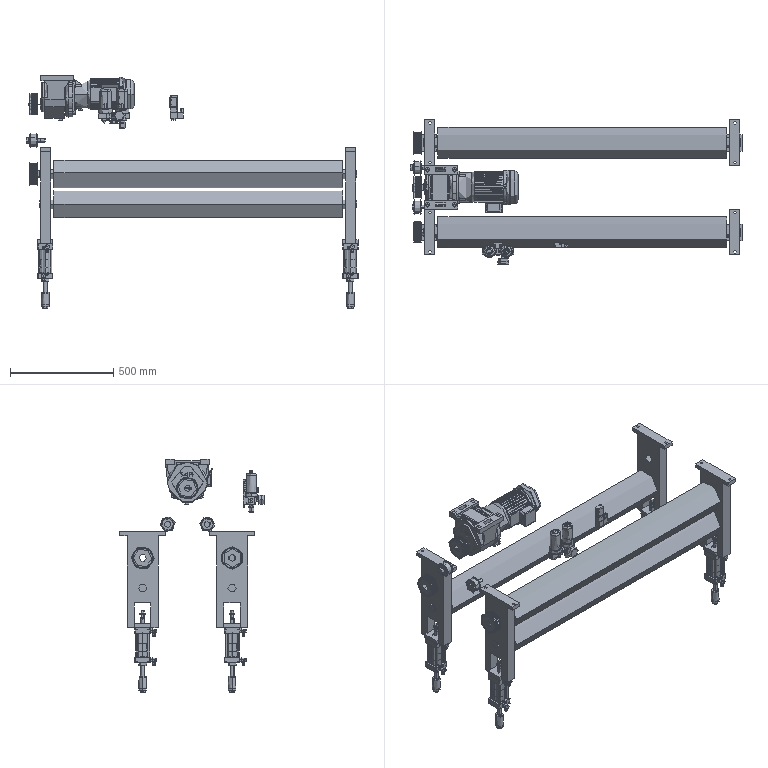Part | SolidWorks | 54 solids | 4760 faces | volume 980797146154168884946852313429228984824106233416722874278836734645215409165302339514138724197191222539980428161043675585091870182479337387475146593540243456 mm3 | cylinder 2200 | plane 1723 | cone 645 | torus 162 | spline 17 | sphere 13 | commonest cylinder face diameters 1.62 x200 100.49 x120 5.14 x118 1.5 x98 0.8 x92 10.6 x86